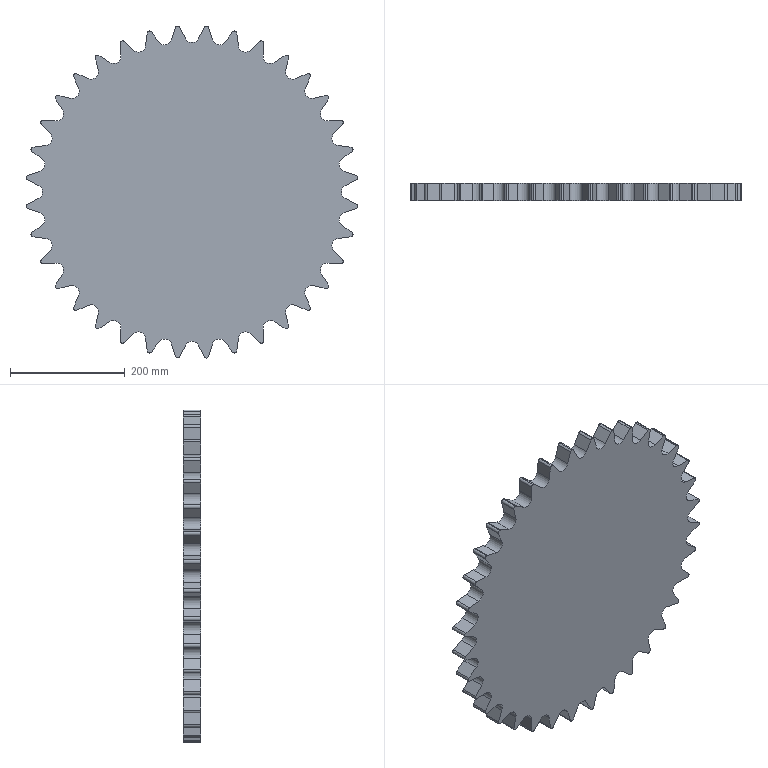Part | SolidWorks | features ICE 2, Extrusion 1 | 1 solid | 173 faces | box 577.823 x 30 x 577.823 mm | volume 6965433 mm3 | cylinder 99 | plane 74 | commonest cylinder face diameters 8 x50 25 x49